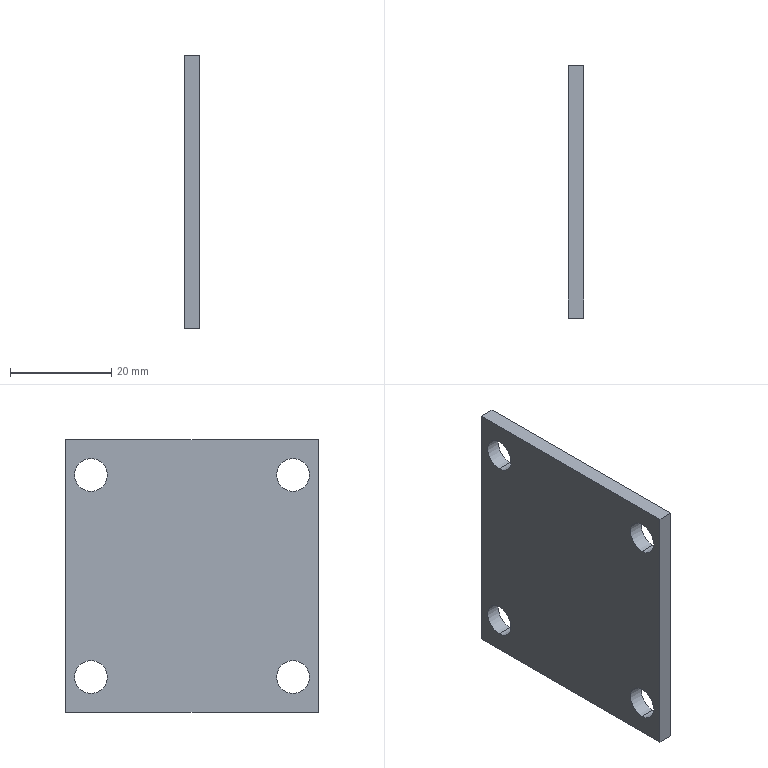Part | STEP file | 09-34 Linear bearing shim | 1 solid | 14 faces | box 3 x 50 x 54 mm | volume 7702 mm3 | cylinder 8 | plane 6 | commonest cylinder face diameters 6.5 x8
STEP:
#1=CARTESIAN_POINT('',(0.,0.,0.));
#2=DIRECTION('',(0.,0.,1.));
#3=DIRECTION('',(1.,0.,0.));
#4=AXIS2_PLACEMENT_3D('',#1,#2,#3);
#5=CARTESIAN_POINT('',(3.,-20.,23.25));
#6=VERTEX_POINT('',#5);
#7=CARTESIAN_POINT('',(0.,-20.,23.25));
#8=VERTEX_POINT('',#7);
#9=CARTESIAN_POINT('',(3.,-20.,23.25));
#10=DIRECTION('',(-1.,0.,0.));
#11=VECTOR('',#10,1.);
#12=LINE('',#9,#11);
#13=CARTESIAN_POINT('',(3.,-20.,20.));
#14=DIRECTION('',(-1.,0.,0.));
#15=DIRECTION('',(0.,0.,1.));
#16=AXIS2_PLACEMENT_3D('',#13,#14,#15);
#17=CYLINDRICAL_SURFACE('',#16,3.25);
#18=CARTESIAN_POINT('',(6.283,0.));
#19=DIRECTION('',(0.,1.));
#20=VECTOR('',#19,1.);
#21=LINE('',#18,#20);
#22=(GEOMETRIC_REPRESENTATION_CONTEXT(2)PARAMETRIC_REPRESENTATION_CONTEXT()REPRESENTATION_CONTEXT('',''));
#23=DEFINITIONAL_REPRESENTATION('',(#21),#22);
#24=PCURVE('',#17,#23);
#25=CARTESIAN_POINT('',(3.,-20.,20.));
#26=DIRECTION('',(-1.,0.,0.));
#27=DIRECTION('',(0.,0.,1.));
#28=AXIS2_PLACEMENT_3D('',#25,#26,#27);
#29=CYLINDRICAL_SURFACE('',#28,3.25);
#30=CARTESIAN_POINT('',(0.,0.));
#31=DIRECTION('',(0.,1.));
#32=VECTOR('',#31,1.);
#33=LINE('',#30,#32);
#34=(GEOMETRIC_REPRESENTATION_CONTEXT(2)PARAMETRIC_REPRESENTATION_CONTEXT()REPRESENTATION_CONTEXT('',''));
#35=DEFINITIONAL_REPRESENTATION('',(#33),#34);
#36=PCURVE('',#29,#35);
#37=SURFACE_CURVE('',#12,(#24,#36),.PCURVE_S1.);
#38=EDGE_CURVE('',#6,#8,#37,.T.);
#39=ORIENTED_EDGE('',*,*,#38,.T.);
#40=CARTESIAN_POINT('',(0.,-20.,16.75));
#41=VERTEX_POINT('',#40);
#42=CARTESIAN_POINT('',(0.,-20.,20.));
#43=DIRECTION('',(-1.,0.,0.));
#44=DIRECTION('',(0.,0.,1.));
#45=AXIS2_PLACEMENT_3D('',#42,#43,#44);
#46=CIRCLE('',#45,3.25);
#47=CARTESIAN_POINT('',(0.,3.));
#48=DIRECTION('',(1.,0.));
#49=VECTOR('',#48,1.);
#50=LINE('',#47,#49);
#51=(GEOMETRIC_REPRESENTATION_CONTEXT(2)PARAMETRIC_REPRESENTATION_CONTEXT()REPRESENTATION_CONTEXT('',''));
#52=DEFINITIONAL_REPRESENTATION('',(#50),#51);
#53=PCURVE('',#17,#52);
#54=CARTESIAN_POINT('',(0.,-25.,27.));
#55=DIRECTION('',(1.,0.,0.));
#56=DIRECTION('',(0.,0.,-1.));
#57=AXIS2_PLACEMENT_3D('',#54,#55,#56);
#58=PLANE('',#57);
#59=CARTESIAN_POINT('',(3.75,5.));
#60=CARTESIAN_POINT('',(3.75,10.629));
#61=CARTESIAN_POINT('',(8.625,7.815));
#62=CARTESIAN_POINT('',(13.5,5.));
#63=CARTESIAN_POINT('',(8.625,2.185));
#64=CARTESIAN_POINT('',(3.75,-0.6292));
#65=CARTESIAN_POINT('',(3.75,5.));
#66=(BOUNDED_CURVE()B_SPLINE_CURVE(2,(#59,#60,#61,#62,#63,#64,#65),.UNSPECIFIED.,.T.,.F.)B_SPLINE_CURVE_WITH_KNOTS((1,2,2,2,2,1),(-2.094,0.,2.094,4.189,6.283,8.378),.UNSPECIFIED.)CURVE()GEOMETRIC_REPRESENTATION_ITEM()RATIONAL_B_SPLINE_CURVE((1.,0.5,1.,0.5,1.,0.5,1.))REPRESENTATION_ITEM(''));
#67=(GEOMETRIC_REPRESENTATION_CONTEXT(2)PARAMETRIC_REPRESENTATION_CONTEXT()REPRESENTATION_CONTEXT('',''));
#68=DEFINITIONAL_REPRESENTATION('',(#66),#67);
#69=PCURVE('',#58,#68);
#70=SURFACE_CURVE('',#46,(#53,#69),.PCURVE_S1.);
#71=EDGE_CURVE('',#41,#8,#70,.T.);
#72=ORIENTED_EDGE('',*,*,#71,.F.);
#73=CARTESIAN_POINT('',(3.,-20.,16.75));
#74=VERTEX_POINT('',#73);
#75=CARTESIAN_POINT('',(3.,-20.,16.75));
#76=DIRECTION('',(-1.,0.,0.));
#77=VECTOR('',#76,1.);
#78=LINE('',#75,#77);
#79=CARTESIAN_POINT('',(3.142,0.));
#80=DIRECTION('',(0.,1.));
#81=VECTOR('',#80,1.);
#82=LINE('',#79,#81);
#83=(GEOMETRIC_REPRESENTATION_CONTEXT(2)PARAMETRIC_REPRESENTATION_CONTEXT()REPRESENTATION_CONTEXT('',''));
#84=DEFINITIONAL_REPRESENTATION('',(#82),#83);
#85=PCURVE('',#17,#84);
#86=CARTESIAN_POINT('',(3.142,0.));
#87=DIRECTION('',(0.,1.));
#88=VECTOR('',#87,1.);
#89=LINE('',#86,#88);
#90=(GEOMETRIC_REPRESENTATION_CONTEXT(2)PARAMETRIC_REPRESENTATION_CONTEXT()REPRESENTATION_CONTEXT('',''));
#91=DEFINITIONAL_REPRESENTATION('',(#89),#90);
#92=PCURVE('',#29,#91);
#93=SURFACE_CURVE('',#78,(#85,#92),.PCURVE_S1.);
#94=EDGE_CURVE('',#74,#41,#93,.T.);
#95=ORIENTED_EDGE('',*,*,#94,.F.);
#96=CARTESIAN_POINT('',(3.,-20.,20.));
#97=DIRECTION('',(1.,0.,0.));
#98=DIRECTION('',(0.,0.,1.));
#99=AXIS2_PLACEMENT_3D('',#96,#97,#98);
#100=CIRCLE('',#99,3.25);
#101=CARTESIAN_POINT('',(6.283,0.));
#102=DIRECTION('',(-1.,0.));
#103=VECTOR('',#102,1.);
#104=LINE('',#101,#103);
#105=(GEOMETRIC_REPRESENTATION_CONTEXT(2)PARAMETRIC_REPRESENTATION_CONTEXT()REPRESENTATION_CONTEXT('',''));
#106=DEFINITIONAL_REPRESENTATION('',(#104),#105);
#107=PCURVE('',#17,#106);
#108=CARTESIAN_POINT('',(3.,-25.,27.));
#109=DIRECTION('',(1.,0.,0.));
#110=DIRECTION('',(0.,0.,-1.));
#111=AXIS2_PLACEMENT_3D('',#108,#109,#110);
#112=PLANE('',#111);
#113=CARTESIAN_POINT('',(7.,5.));
#114=DIRECTION('',(-1.,0.));
#115=AXIS2_PLACEMENT_2D('',#113,#114);
#116=CIRCLE('',#115,3.25);
#117=(GEOMETRIC_REPRESENTATION_CONTEXT(2)PARAMETRIC_REPRESENTATION_CONTEXT()REPRESENTATION_CONTEXT('',''));
#118=DEFINITIONAL_REPRESENTATION('',(#116),#117);
#119=PCURVE('',#112,#118);
#120=SURFACE_CURVE('',#100,(#107,#119),.PCURVE_S1.);
#121=EDGE_CURVE('',#6,#74,#120,.T.);
#122=ORIENTED_EDGE('',*,*,#121,.F.);
#123=EDGE_LOOP('',(#39,#72,#95,#122));
#124=FACE_BOUND('',#123,.F.);
#125=ADVANCED_FACE('',(#124),#17,.F.);
#126=CARTESIAN_POINT('',(3.,20.,23.25));
#127=VERTEX_POINT('',#126);
#128=CARTESIAN_POINT('',(0.,20.,23.25));
#129=VERTEX_POINT('',#128);
#130=CARTESIAN_POINT('',(3.,20.,23.25));
#131=DIRECTION('',(-1.,0.,0.));
#132=VECTOR('',#131,1.);
#133=LINE('',#130,#132);
#134=CARTESIAN_POINT('',(3.,20.,20.));
#135=DIRECTION('',(-1.,0.,0.));
#136=DIRECTION('',(0.,0.,1.));
#137=AXIS2_PLACEMENT_3D('',#134,#135,#136);
#138=CYLINDRICAL_SURFACE('',#137,3.25);
#139=CARTESIAN_POINT('',(6.283,0.));
#140=DIRECTION('',(0.,1.));
#141=VECTOR('',#140,1.);
#142=LINE('',#139,#141);
#143=(GEOMETRIC_REPRESENTATION_CONTEXT(2)PARAMETRIC_REPRESENTATION_CONTEXT()REPRESENTATION_CONTEXT('',''));
#144=DEFINITIONAL_REPRESENTATION('',(#142),#143);
#145=PCURVE('',#138,#144);
#146=CARTESIAN_POINT('',(3.,20.,20.));
#147=DIRECTION('',(-1.,0.,0.));
#148=DIRECTION('',(0.,0.,1.));
#149=AXIS2_PLACEMENT_3D('',#146,#147,#148);
#150=CYLINDRICAL_SURFACE('',#149,3.25);
#151=CARTESIAN_POINT('',(0.,0.));
#152=DIRECTION('',(0.,1.));
#153=VECTOR('',#152,1.);
#154=LINE('',#151,#153);
#155=(GEOMETRIC_REPRESENTATION_CONTEXT(2)PARAMETRIC_REPRESENTATION_CONTEXT()REPRESENTATION_CONTEXT('',''));
#156=DEFINITIONAL_REPRESENTATION('',(#154),#155);
#157=PCURVE('',#150,#156);
#158=SURFACE_CURVE('',#133,(#145,#157),.PCURVE_S1.);
#159=EDGE_CURVE('',#127,#129,#158,.T.);
#160=ORIENTED_EDGE('',*,*,#159,.T.);
#161=CARTESIAN_POINT('',(0.,20.,16.75));
#162=VERTEX_POINT('',#161);
#163=CARTESIAN_POINT('',(0.,20.,20.));
#164=DIRECTION('',(-1.,0.,0.));
#165=DIRECTION('',(0.,0.,1.));
#166=AXIS2_PLACEMENT_3D('',#163,#164,#165);
#167=CIRCLE('',#166,3.25);
#168=CARTESIAN_POINT('',(0.,3.));
#169=DIRECTION('',(1.,0.));
#170=VECTOR('',#169,1.);
#171=LINE('',#168,#170);
#172=(GEOMETRIC_REPRESENTATION_CONTEXT(2)PARAMETRIC_REPRESENTATION_CONTEXT()REPRESENTATION_CONTEXT('',''));
#173=DEFINITIONAL_REPRESENTATION('',(#171),#172);
#174=PCURVE('',#138,#173);
#175=CARTESIAN_POINT('',(3.75,45.));
#176=CARTESIAN_POINT('',(3.75,50.629));
#177=CARTESIAN_POINT('',(8.625,47.815));
#178=CARTESIAN_POINT('',(13.5,45.));
#179=CARTESIAN_POINT('',(8.625,42.185));
#180=CARTESIAN_POINT('',(3.75,39.371));
#181=CARTESIAN_POINT('',(3.75,45.));
#182=(BOUNDED_CURVE()B_SPLINE_CURVE(2,(#175,#176,#177,#178,#179,#180,#181),.UNSPECIFIED.,.T.,.F.)B_SPLINE_CURVE_WITH_KNOTS((1,2,2,2,2,1),(-2.094,0.,2.094,4.189,6.283,8.378),.UNSPECIFIED.)CURVE()GEOMETRIC_REPRESENTATION_ITEM()RATIONAL_B_SPLINE_CURVE((1.,0.5,1.,0.5,1.,0.5,1.))REPRESENTATION_ITEM(''));
#183=(GEOMETRIC_REPRESENTATION_CONTEXT(2)PARAMETRIC_REPRESENTATION_CONTEXT()REPRESENTATION_CONTEXT('',''));
#184=DEFINITIONAL_REPRESENTATION('',(#182),#183);
#185=PCURVE('',#58,#184);
#186=SURFACE_CURVE('',#167,(#174,#185),.PCURVE_S1.);
#187=EDGE_CURVE('',#162,#129,#186,.T.);
#188=ORIENTED_EDGE('',*,*,#187,.F.);
#189=CARTESIAN_POINT('',(3.,20.,16.75));
#190=VERTEX_POINT('',#189);
#191=CARTESIAN_POINT('',(3.,20.,16.75));
#192=DIRECTION('',(-1.,0.,0.));
#193=VECTOR('',#192,1.);
#194=LINE('',#191,#193);
#195=CARTESIAN_POINT('',(3.142,0.));
#196=DIRECTION('',(0.,1.));
#197=VECTOR('',#196,1.);
#198=LINE('',#195,#197);
#199=(GEOMETRIC_REPRESENTATION_CONTEXT(2)PARAMETRIC_REPRESENTATION_CONTEXT()REPRESENTATION_CONTEXT('',''));
#200=DEFINITIONAL_REPRESENTATION('',(#198),#199);
#201=PCURVE('',#138,#200);
#202=CARTESIAN_POINT('',(3.142,0.));
#203=DIRECTION('',(0.,1.));
#204=VECTOR('',#203,1.);
#205=LINE('',#202,#204);
#206=(GEOMETRIC_REPRESENTATION_CONTEXT(2)PARAMETRIC_REPRESENTATION_CONTEXT()REPRESENTATION_CONTEXT('',''));
#207=DEFINITIONAL_REPRESENTATION('',(#205),#206);
#208=PCURVE('',#150,#207);
#209=SURFACE_CURVE('',#194,(#201,#208),.PCURVE_S1.);
#210=EDGE_CURVE('',#190,#162,#209,.T.);
#211=ORIENTED_EDGE('',*,*,#210,.F.);
#212=CARTESIAN_POINT('',(3.,20.,20.));
#213=DIRECTION('',(-1.,0.,0.));
#214=DIRECTION('',(0.,0.,1.));
#215=AXIS2_PLACEMENT_3D('',#212,#213,#214);
#216=CIRCLE('',#215,3.25);
#217=CARTESIAN_POINT('',(0.,0.));
#218=DIRECTION('',(1.,0.));
#219=VECTOR('',#218,1.);
#220=LINE('',#217,#219);
#221=(GEOMETRIC_REPRESENTATION_CONTEXT(2)PARAMETRIC_REPRESENTATION_CONTEXT()REPRESENTATION_CONTEXT('',''));
#222=DEFINITIONAL_REPRESENTATION('',(#220),#221);
#223=PCURVE('',#138,#222);
#224=CARTESIAN_POINT('',(3.75,45.));
#225=CARTESIAN_POINT('',(3.75,50.629));
#226=CARTESIAN_POINT('',(8.625,47.815));
#227=CARTESIAN_POINT('',(13.5,45.));
#228=CARTESIAN_POINT('',(8.625,42.185));
#229=CARTESIAN_POINT('',(3.75,39.371));
#230=CARTESIAN_POINT('',(3.75,45.));
#231=(BOUNDED_CURVE()B_SPLINE_CURVE(2,(#224,#225,#226,#227,#228,#229,#230),.UNSPECIFIED.,.T.,.F.)B_SPLINE_CURVE_WITH_KNOTS((1,2,2,2,2,1),(-2.094,0.,2.094,4.189,6.283,8.378),.UNSPECIFIED.)CURVE()GEOMETRIC_REPRESENTATION_ITEM()RATIONAL_B_SPLINE_CURVE((1.,0.5,1.,0.5,1.,0.5,1.))REPRESENTATION_ITEM(''));
#232=(GEOMETRIC_REPRESENTATION_CONTEXT(2)PARAMETRIC_REPRESENTATION_CONTEXT()REPRESENTATION_CONTEXT('',''));
#233=DEFINITIONAL_REPRESENTATION('',(#231),#232);
#234=PCURVE('',#112,#233);
#235=SURFACE_CURVE('',#216,(#223,#234),.PCURVE_S1.);
#236=EDGE_CURVE('',#190,#127,#235,.T.);
#237=ORIENTED_EDGE('',*,*,#236,.T.);
#238=EDGE_LOOP('',(#160,#188,#211,#237));
#239=FACE_BOUND('',#238,.F.);
#240=ADVANCED_FACE('',(#239),#138,.F.);
#241=CARTESIAN_POINT('',(3.,20.,-16.75));
#242=VERTEX_POINT('',#241);
#243=CARTESIAN_POINT('',(0.,20.,-16.75));
#244=VERTEX_POINT('',#243);
#245=CARTESIAN_POINT('',(3.,20.,-16.75));
#246=DIRECTION('',(-1.,0.,0.));
#247=VECTOR('',#246,1.);
#248=LINE('',#245,#247);
#249=CARTESIAN_POINT('',(3.,20.,-20.));
#250=DIRECTION('',(-1.,0.,0.));
#251=DIRECTION('',(0.,0.,1.));
#252=AXIS2_PLACEMENT_3D('',#249,#250,#251);
#253=CYLINDRICAL_SURFACE('',#252,3.25);
#254=CARTESIAN_POINT('',(6.283,0.));
#255=DIRECTION('',(0.,1.));
#256=VECTOR('',#255,1.);
#257=LINE('',#254,#256);
#258=(GEOMETRIC_REPRESENTATION_CONTEXT(2)PARAMETRIC_REPRESENTATION_CONTEXT()REPRESENTATION_CONTEXT('',''));
#259=DEFINITIONAL_REPRESENTATION('',(#257),#258);
#260=PCURVE('',#253,#259);
#261=CARTESIAN_POINT('',(3.,20.,-20.));
#262=DIRECTION('',(-1.,0.,0.));
#263=DIRECTION('',(0.,0.,1.));
#264=AXIS2_PLACEMENT_3D('',#261,#262,#263);
#265=CYLINDRICAL_SURFACE('',#264,3.25);
#266=CARTESIAN_POINT('',(0.,0.));
#267=DIRECTION('',(0.,1.));
#268=VECTOR('',#267,1.);
#269=LINE('',#266,#268);
#270=(GEOMETRIC_REPRESENTATION_CONTEXT(2)PARAMETRIC_REPRESENTATION_CONTEXT()REPRESENTATION_CONTEXT('',''));
#271=DEFINITIONAL_REPRESENTATION('',(#269),#270);
#272=PCURVE('',#265,#271);
#273=SURFACE_CURVE('',#248,(#260,#272),.PCURVE_S1.);
#274=EDGE_CURVE('',#242,#244,#273,.T.);
#275=ORIENTED_EDGE('',*,*,#274,.T.);
#276=CARTESIAN_POINT('',(0.,20.,-23.25));
#277=VERTEX_POINT('',#276);
#278=CARTESIAN_POINT('',(0.,20.,-20.));
#279=DIRECTION('',(-1.,0.,0.));
#280=DIRECTION('',(0.,0.,1.));
#281=AXIS2_PLACEMENT_3D('',#278,#279,#280);
#282=CIRCLE('',#281,3.25);
#283=CARTESIAN_POINT('',(0.,3.));
#284=DIRECTION('',(1.,0.));
#285=VECTOR('',#284,1.);
#286=LINE('',#283,#285);
#287=(GEOMETRIC_REPRESENTATION_CONTEXT(2)PARAMETRIC_REPRESENTATION_CONTEXT()REPRESENTATION_CONTEXT('',''));
#288=DEFINITIONAL_REPRESENTATION('',(#286),#287);
#289=PCURVE('',#253,#288);
#290=CARTESIAN_POINT('',(43.75,45.));
#291=CARTESIAN_POINT('',(43.75,50.629));
#292=CARTESIAN_POINT('',(48.625,47.815));
#293=CARTESIAN_POINT('',(53.5,45.));
#294=CARTESIAN_POINT('',(48.625,42.185));
#295=CARTESIAN_POINT('',(43.75,39.371));
#296=CARTESIAN_POINT('',(43.75,45.));
#297=(BOUNDED_CURVE()B_SPLINE_CURVE(2,(#290,#291,#292,#293,#294,#295,#296),.UNSPECIFIED.,.T.,.F.)B_SPLINE_CURVE_WITH_KNOTS((1,2,2,2,2,1),(-2.094,0.,2.094,4.189,6.283,8.378),.UNSPECIFIED.)CURVE()GEOMETRIC_REPRESENTATION_ITEM()RATIONAL_B_SPLINE_CURVE((1.,0.5,1.,0.5,1.,0.5,1.))REPRESENTATION_ITEM(''));
#298=(GEOMETRIC_REPRESENTATION_CONTEXT(2)PARAMETRIC_REPRESENTATION_CONTEXT()REPRESENTATION_CONTEXT('',''));
#299=DEFINITIONAL_REPRESENTATION('',(#297),#298);
#300=PCURVE('',#58,#299);
#301=SURFACE_CURVE('',#282,(#289,#300),.PCURVE_S1.);
#302=EDGE_CURVE('',#277,#244,#301,.T.);
#303=ORIENTED_EDGE('',*,*,#302,.F.);
#304=CARTESIAN_POINT('',(3.,20.,-23.25));
#305=VERTEX_POINT('',#304);
#306=CARTESIAN_POINT('',(3.,20.,-23.25));
#307=DIRECTION('',(-1.,0.,0.));
#308=VECTOR('',#307,1.);
#309=LINE('',#306,#308);
#310=CARTESIAN_POINT('',(3.142,0.));
#311=DIRECTION('',(0.,1.));
#312=VECTOR('',#311,1.);
#313=LINE('',#310,#312);
#314=(GEOMETRIC_REPRESENTATION_CONTEXT(2)PARAMETRIC_REPRESENTATION_CONTEXT()REPRESENTATION_CONTEXT('',''));
#315=DEFINITIONAL_REPRESENTATION('',(#313),#314);
#316=PCURVE('',#253,#315);
#317=CARTESIAN_POINT('',(3.142,0.));
#318=DIRECTION('',(0.,1.));
#319=VECTOR('',#318,1.);
#320=LINE('',#317,#319);
#321=(GEOMETRIC_REPRESENTATION_CONTEXT(2)PARAMETRIC_REPRESENTATION_CONTEXT()REPRESENTATION_CONTEXT('',''));
#322=DEFINITIONAL_REPRESENTATION('',(#320),#321);
#323=PCURVE('',#265,#322);
#324=SURFACE_CURVE('',#309,(#316,#323),.PCURVE_S1.);
#325=EDGE_CURVE('',#305,#277,#324,.T.);
#326=ORIENTED_EDGE('',*,*,#325,.F.);
#327=CARTESIAN_POINT('',(3.,20.,-20.));
#328=DIRECTION('',(-1.,0.,0.));
#329=DIRECTION('',(0.,0.,1.));
#330=AXIS2_PLACEMENT_3D('',#327,#328,#329);
#331=CIRCLE('',#330,3.25);
#332=CARTESIAN_POINT('',(0.,0.));
#333=DIRECTION('',(1.,0.));
#334=VECTOR('',#333,1.);
#335=LINE('',#332,#334);
#336=(GEOMETRIC_REPRESENTATION_CONTEXT(2)PARAMETRIC_REPRESENTATION_CONTEXT()REPRESENTATION_CONTEXT('',''));
#337=DEFINITIONAL_REPRESENTATION('',(#335),#336);
#338=PCURVE('',#253,#337);
#339=CARTESIAN_POINT('',(43.75,45.));
#340=CARTESIAN_POINT('',(43.75,50.629));
#341=CARTESIAN_POINT('',(48.625,47.815));
#342=CARTESIAN_POINT('',(53.5,45.));
#343=CARTESIAN_POINT('',(48.625,42.185));
#344=CARTESIAN_POINT('',(43.75,39.371));
#345=CARTESIAN_POINT('',(43.75,45.));
#346=(BOUNDED_CURVE()B_SPLINE_CURVE(2,(#339,#340,#341,#342,#343,#344,#345),.UNSPECIFIED.,.T.,.F.)B_SPLINE_CURVE_WITH_KNOTS((1,2,2,2,2,1),(-2.094,0.,2.094,4.189,6.283,8.378),.UNSPECIFIED.)CURVE()GEOMETRIC_REPRESENTATION_ITEM()RATIONAL_B_SPLINE_CURVE((1.,0.5,1.,0.5,1.,0.5,1.))REPRESENTATION_ITEM(''));
#347=(GEOMETRIC_REPRESENTATION_CONTEXT(2)PARAMETRIC_REPRESENTATION_CONTEXT()REPRESENTATION_CONTEXT('',''));
#348=DEFINITIONAL_REPRESENTATION('',(#346),#347);
#349=PCURVE('',#112,#348);
#350=SURFACE_CURVE('',#331,(#338,#349),.PCURVE_S1.);
#351=EDGE_CURVE('',#305,#242,#350,.T.);
#352=ORIENTED_EDGE('',*,*,#351,.T.);
#353=EDGE_LOOP('',(#275,#303,#326,#352));
#354=FACE_BOUND('',#353,.F.);
#355=ADVANCED_FACE('',(#354),#253,.F.);
#356=CARTESIAN_POINT('',(3.,-20.,-16.75));
#357=VERTEX_POINT('',#356);
#358=CARTESIAN_POINT('',(0.,-20.,-16.75));
#359=VERTEX_POINT('',#358);
#360=CARTESIAN_POINT('',(3.,-20.,-16.75));
#361=DIRECTION('',(-1.,0.,0.));
#362=VECTOR('',#361,1.);
#363=LINE('',#360,#362);
#364=CARTESIAN_POINT('',(3.,-20.,-20.));
#365=DIRECTION('',(-1.,0.,0.));
#366=DIRECTION('',(0.,0.,1.));
#367=AXIS2_PLACEMENT_3D('',#364,#365,#366);
#368=CYLINDRICAL_SURFACE('',#367,3.25);
#369=CARTESIAN_POINT('',(6.283,0.));
#370=DIRECTION('',(0.,1.));
#371=VECTOR('',#370,1.);
#372=LINE('',#369,#371);
#373=(GEOMETRIC_REPRESENTATION_CONTEXT(2)PARAMETRIC_REPRESENTATION_CONTEXT()REPRESENTATION_CONTEXT('',''));
#374=DEFINITIONAL_REPRESENTATION('',(#372),#373);
#375=PCURVE('',#368,#374);
#376=CARTESIAN_POINT('',(3.,-20.,-20.));
#377=DIRECTION('',(-1.,0.,0.));
#378=DIRECTION('',(0.,0.,1.));
#379=AXIS2_PLACEMENT_3D('',#376,#377,#378);
#380=CYLINDRICAL_SURFACE('',#379,3.25);
#381=CARTESIAN_POINT('',(0.,0.));
#382=DIRECTION('',(0.,1.));
#383=VECTOR('',#382,1.);
#384=LINE('',#381,#383);
#385=(GEOMETRIC_REPRESENTATION_CONTEXT(2)PARAMETRIC_REPRESENTATION_CONTEXT()REPRESENTATION_CONTEXT('',''));
#386=DEFINITIONAL_REPRESENTATION('',(#384),#385);
#387=PCURVE('',#380,#386);
#388=SURFACE_CURVE('',#363,(#375,#387),.PCURVE_S1.);
#389=EDGE_CURVE('',#357,#359,#388,.T.);
#390=ORIENTED_EDGE('',*,*,#389,.T.);
#391=CARTESIAN_POINT('',(0.,-20.,-23.25));
#392=VERTEX_POINT('',#391);
#393=CARTESIAN_POINT('',(0.,-20.,-20.));
#394=DIRECTION('',(-1.,0.,0.));
#395=DIRECTION('',(0.,0.,1.));
#396=AXIS2_PLACEMENT_3D('',#393,#394,#395);
#397=CIRCLE('',#396,3.25);
#398=CARTESIAN_POINT('',(0.,3.));
#399=DIRECTION('',(1.,0.));
#400=VECTOR('',#399,1.);
#401=LINE('',#398,#400);
#402=(GEOMETRIC_REPRESENTATION_CONTEXT(2)PARAMETRIC_REPRESENTATION_CONTEXT()REPRESENTATION_CONTEXT('',''));
#403=DEFINITIONAL_REPRESENTATION('',(#401),#402);
#404=PCURVE('',#368,#403);
#405=CARTESIAN_POINT('',(43.75,5.));
#406=CARTESIAN_POINT('',(43.75,10.629));
#407=CARTESIAN_POINT('',(48.625,7.815));
#408=CARTESIAN_POINT('',(53.5,5.));
#409=CARTESIAN_POINT('',(48.625,2.185));
#410=CARTESIAN_POINT('',(43.75,-0.6292));
#411=CARTESIAN_POINT('',(43.75,5.));
#412=(BOUNDED_CURVE()B_SPLINE_CURVE(2,(#405,#406,#407,#408,#409,#410,#411),.UNSPECIFIED.,.T.,.F.)B_SPLINE_CURVE_WITH_KNOTS((1,2,2,2,2,1),(-2.094,0.,2.094,4.189,6.283,8.378),.UNSPECIFIED.)CURVE()GEOMETRIC_REPRESENTATION_ITEM()RATIONAL_B_SPLINE_CURVE((1.,0.5,1.,0.5,1.,0.5,1.))REPRESENTATION_ITEM(''));
#413=(GEOMETRIC_REPRESENTATION_CONTEXT(2)PARAMETRIC_REPRESENTATION_CONTEXT()REPRESENTATION_CONTEXT('',''));
#414=DEFINITIONAL_REPRESENTATION('',(#412),#413);
#415=PCURVE('',#58,#414);
#416=SURFACE_CURVE('',#397,(#404,#415),.PCURVE_S1.);
#417=EDGE_CURVE('',#392,#359,#416,.T.);
#418=ORIENTED_EDGE('',*,*,#417,.F.);
#419=CARTESIAN_POINT('',(3.,-20.,-23.25));
#420=VERTEX_POINT('',#419);
#421=CARTESIAN_POINT('',(3.,-20.,-23.25));
#422=DIRECTION('',(-1.,0.,0.));
#423=VECTOR('',#422,1.);
#424=LINE('',#421,#423);
#425=CARTESIAN_POINT('',(3.142,0.));
#426=DIRECTION('',(0.,1.));
#427=VECTOR('',#426,1.);
#428=LINE('',#425,#427);
#429=(GEOMETRIC_REPRESENTATION_CONTEXT(2)PARAMETRIC_REPRESENTATION_CONTEXT()REPRESENTATION_CONTEXT('',''));
#430=DEFINITIONAL_REPRESENTATION('',(#428),#429);
#431=PCURVE('',#368,#430);
#432=CARTESIAN_POINT('',(3.142,0.));
#433=DIRECTION('',(0.,1.));
#434=VECTOR('',#433,1.);
#435=LINE('',#432,#434);
#436=(GEOMETRIC_REPRESENTATION_CONTEXT(2)PARAMETRIC_REPRESENTATION_CONTEXT()REPRESENTATION_CONTEXT('',''));
#437=DEFINITIONAL_REPRESENTATION('',(#435),#436);
#438=PCURVE('',#380,#437);
#439=SURFACE_CURVE('',#424,(#431,#438),.PCURVE_S1.);
#440=EDGE_CURVE('',#420,#392,#439,.T.);
#441=ORIENTED_EDGE('',*,*,#440,.F.);
#442=CARTESIAN_POINT('',(3.,-20.,-20.));
#443=DIRECTION('',(-1.,0.,0.));
#444=DIRECTION('',(0.,0.,1.));
#445=AXIS2_PLACEMENT_3D('',#442,#443,#444);
#446=CIRCLE('',#445,3.25);
#447=CARTESIAN_POINT('',(0.,0.));
#448=DIRECTION('',(1.,0.));
#449=VECTOR('',#448,1.);
#450=LINE('',#447,#449);
#451=(GEOMETRIC_REPRESENTATION_CONTEXT(2)PARAMETRIC_REPRESENTATION_CONTEXT()REPRESENTATION_CONTEXT('',''));
#452=DEFINITIONAL_REPRESENTATION('',(#450),#451);
#453=PCURVE('',#368,#452);
#454=CARTESIAN_POINT('',(43.75,5.));
#455=CARTESIAN_POINT('',(43.75,10.629));
#456=CARTESIAN_POINT('',(48.625,7.815));
#457=CARTESIAN_POINT('',(53.5,5.));
#458=CARTESIAN_POINT('',(48.625,2.185));
#459=CARTESIAN_POINT('',(43.75,-0.6292));
#460=CARTESIAN_POINT('',(43.75,5.));
#461=(BOUNDED_CURVE()B_SPLINE_CURVE(2,(#454,#455,#456,#457,#458,#459,#460),.UNSPECIFIED.,.T.,.F.)B_SPLINE_CURVE_WITH_KNOTS((1,2,2,2,2,1),(-2.094,0.,2.094,4.189,6.283,8.378),.UNSPECIFIED.)CURVE()GEOMETRIC_REPRESENTATION_ITEM()RATIONAL_B_SPLINE_CURVE((1.,0.5,1.,0.5,1.,0.5,1.))REPRESENTATION_ITEM(''));
#462=(GEOMETRIC_REPRESENTATION_CONTEXT(2)PARAMETRIC_REPRESENTATION_CONTEXT()REPRESENTATION_CONTEXT('',''));
#463=DEFINITIONAL_REPRESENTATION('',(#461),#462);
#464=PCURVE('',#112,#463);
#465=SURFACE_CURVE('',#446,(#453,#464),.PCURVE_S1.);
#466=EDGE_CURVE('',#420,#357,#465,.T.);
#467=ORIENTED_EDGE('',*,*,#466,.T.);
#468=EDGE_LOOP('',(#390,#418,#441,#467));
#469=FACE_BOUND('',#468,.F.);
#470=ADVANCED_FACE('',(#469),#368,.F.);
#471=CARTESIAN_POINT('',(0.,-20.,20.));
#472=DIRECTION('',(-1.,0.,0.));
#473=DIRECTION('',(0.,0.,1.));
#474=AXIS2_PLACEMENT_3D('',#471,#472,#473);
#475=CIRCLE('',#474,3.25);
#476=CARTESIAN_POINT('',(0.,3.));
#477=DIRECTION('',(1.,0.));
#478=VECTOR('',#477,1.);
#479=LINE('',#476,#478);
#480=(GEOMETRIC_REPRESENTATION_CONTEXT(2)PARAMETRIC_REPRESENTATION_CONTEXT()REPRESENTATION_CONTEXT('',''));
#481=DEFINITIONAL_REPRESENTATION('',(#479),#480);
#482=PCURVE('',#29,#481);
#483=CARTESIAN_POINT('',(3.75,5.));
#484=CARTESIAN_POINT('',(3.75,10.629));
#485=CARTESIAN_POINT('',(8.625,7.815));
#486=CARTESIAN_POINT('',(13.5,5.));
#487=CARTESIAN_POINT('',(8.625,2.185));
#488=CARTESIAN_POINT('',(3.75,-0.6292));
#489=CARTESIAN_POINT('',(3.75,5.));
#490=(BOUNDED_CURVE()B_SPLINE_CURVE(2,(#483,#484,#485,#486,#487,#488,#489),.UNSPECIFIED.,.T.,.F.)B_SPLINE_CURVE_WITH_KNOTS((1,2,2,2,2,1),(-2.094,0.,2.094,4.189,6.283,8.378),.UNSPECIFIED.)CURVE()GEOMETRIC_REPRESENTATION_ITEM()RATIONAL_B_SPLINE_CURVE((1.,0.5,1.,0.5,1.,0.5,1.))REPRESENTATION_ITEM(''));
#491=(GEOMETRIC_REPRESENTATION_CONTEXT(2)PARAMETRIC_REPRESENTATION_CONTEXT()REPRESENTATION_CONTEXT('',''));
#492=DEFINITIONAL_REPRESENTATION('',(#490),#491);
#493=PCURVE('',#58,#492);
#494=SURFACE_CURVE('',#475,(#482,#493),.PCURVE_S1.);
#495=EDGE_CURVE('',#8,#41,#494,.T.);
#496=ORIENTED_EDGE('',*,*,#495,.F.);
#497=ORIENTED_EDGE('',*,*,#38,.F.);
#498=CARTESIAN_POINT('',(3.,-20.,20.));
#499=DIRECTION('',(1.,0.,0.));
#500=DIRECTION('',(0.,0.,1.));
#501=AXIS2_PLACEMENT_3D('',#498,#499,#500);
#502=CIRCLE('',#501,3.25);
#503=CARTESIAN_POINT('',(6.283,0.));
#504=DIRECTION('',(-1.,0.));
#505=VECTOR('',#504,1.);
#506=LINE('',#503,#505);
#507=(GEOMETRIC_REPRESENTATION_CONTEXT(2)PARAMETRIC_REPRESENTATION_CONTEXT()REPRESENTATION_CONTEXT('',''));
#508=DEFINITIONAL_REPRESENTATION('',(#506),#507);
#509=PCURVE('',#29,#508);
#510=CARTESIAN_POINT('',(7.,5.));
#511=DIRECTION('',(-1.,0.));
#512=AXIS2_PLACEMENT_2D('',#510,#511);
#513=CIRCLE('',#512,3.25);
#514=(GEOMETRIC_REPRESENTATION_CONTEXT(2)PARAMETRIC_REPRESENTATION_CONTEXT()REPRESENTATION_CONTEXT('',''));
#515=DEFINITIONAL_REPRESENTATION('',(#513),#514);
#516=PCURVE('',#112,#515);
#517=SURFACE_CURVE('',#502,(#509,#516),.PCURVE_S1.);
#518=EDGE_CURVE('',#74,#6,#517,.T.);
#519=ORIENTED_EDGE('',*,*,#518,.F.);
#520=ORIENTED_EDGE('',*,*,#94,.T.);
#521=EDGE_LOOP('',(#496,#497,#519,#520));
#522=FACE_BOUND('',#521,.F.);
#523=ADVANCED_FACE('',(#522),#29,.F.);
#524=ORIENTED_EDGE('',*,*,#495,.F.);
#525=ORIENTED_EDGE('',*,*,#71,.F.);
#526=EDGE_LOOP('',(#524,#525));
#527=FACE_BOUND('',#526,.T.);
#528=CARTESIAN_POINT('',(0.,20.,20.));
#529=DIRECTION('',(-1.,0.,0.));
#530=DIRECTION('',(0.,0.,1.));
#531=AXIS2_PLACEMENT_3D('',#528,#529,#530);
#532=CIRCLE('',#531,3.25);
#533=CARTESIAN_POINT('',(3.75,45.));
#534=CARTESIAN_POINT('',(3.75,50.629));
#535=CARTESIAN_POINT('',(8.625,47.815));
#536=CARTESIAN_POINT('',(13.5,45.));
#537=CARTESIAN_POINT('',(8.625,42.185));
#538=CARTESIAN_POINT('',(3.75,39.371));
#539=CARTESIAN_POINT('',(3.75,45.));
#540=(BOUNDED_CURVE()B_SPLINE_CURVE(2,(#533,#534,#535,#536,#537,#538,#539),.UNSPECIFIED.,.T.,.F.)B_SPLINE_CURVE_WITH_KNOTS((1,2,2,2,2,1),(-2.094,0.,2.094,4.189,6.283,8.378),.UNSPECIFIED.)CURVE()GEOMETRIC_REPRESENTATION_ITEM()RATIONAL_B_SPLINE_CURVE((1.,0.5,1.,0.5,1.,0.5,1.))REPRESENTATION_ITEM(''));
#541=(GEOMETRIC_REPRESENTATION_CONTEXT(2)PARAMETRIC_REPRESENTATION_CONTEXT()REPRESENTATION_CONTEXT('',''));
#542=DEFINITIONAL_REPRESENTATION('',(#540),#541);
#543=PCURVE('',#58,#542);
#544=CARTESIAN_POINT('',(0.,3.));
#545=DIRECTION('',(1.,0.));
#546=VECTOR('',#545,1.);
#547=LINE('',#544,#546);
#548=(GEOMETRIC_REPRESENTATION_CONTEXT(2)PARAMETRIC_REPRESENTATION_CONTEXT()REPRESENTATION_CONTEXT('',''));
#549=DEFINITIONAL_REPRESENTATION('',(#547),#548);
#550=PCURVE('',#150,#549);
#551=SURFACE_CURVE('',#532,(#543,#550),.PCURVE_S1.);
#552=EDGE_CURVE('',#129,#162,#551,.T.);
#553=ORIENTED_EDGE('',*,*,#552,.F.);
#554=ORIENTED_EDGE('',*,*,#187,.F.);
#555=EDGE_LOOP('',(#553,#554));
#556=FACE_BOUND('',#555,.T.);
#557=CARTESIAN_POINT('',(0.,20.,-20.));
#558=DIRECTION('',(-1.,0.,0.));
#559=DIRECTION('',(0.,0.,1.));
#560=AXIS2_PLACEMENT_3D('',#557,#558,#559);
#561=CIRCLE('',#560,3.25);
#562=CARTESIAN_POINT('',(43.75,45.));
#563=CARTESIAN_POINT('',(43.75,50.629));
#564=CARTESIAN_POINT('',(48.625,47.815));
#565=CARTESIAN_POINT('',(53.5,45.));
#566=CARTESIAN_POINT('',(48.625,42.185));
#567=CARTESIAN_POINT('',(43.75,39.371));
#568=CARTESIAN_POINT('',(43.75,45.));
#569=(BOUNDED_CURVE()B_SPLINE_CURVE(2,(#562,#563,#564,#565,#566,#567,#568),.UNSPECIFIED.,.T.,.F.)B_SPLINE_CURVE_WITH_KNOTS((1,2,2,2,2,1),(-2.094,0.,2.094,4.189,6.283,8.378),.UNSPECIFIED.)CURVE()GEOMETRIC_REPRESENTATION_ITEM()RATIONAL_B_SPLINE_CURVE((1.,0.5,1.,0.5,1.,0.5,1.))REPRESENTATION_ITEM(''));
#570=(GEOMETRIC_REPRESENTATION_CONTEXT(2)PARAMETRIC_REPRESENTATION_CONTEXT()REPRESENTATION_CONTEXT('',''));
#571=DEFINITIONAL_REPRESENTATION('',(#569),#570);
#572=PCURVE('',#58,#571);
#573=CARTESIAN_POINT('',(0.,3.));
#574=DIRECTION('',(1.,0.));
#575=VECTOR('',#574,1.);
#576=LINE('',#573,#575);
#577=(GEOMETRIC_REPRESENTATION_CONTEXT(2)PARAMETRIC_REPRESENTATION_CONTEXT()REPRESENTATION_CONTEXT('',''));
#578=DEFINITIONAL_REPRESENTATION('',(#576),#577);
#579=PCURVE('',#265,#578);
#580=SURFACE_CURVE('',#561,(#572,#579),.PCURVE_S1.);
#581=EDGE_CURVE('',#244,#277,#580,.T.);
#582=ORIENTED_EDGE('',*,*,#581,.F.);
#583=ORIENTED_EDGE('',*,*,#302,.F.);
#584=EDGE_LOOP('',(#582,#583));
#585=FACE_BOUND('',#584,.T.);
#586=CARTESIAN_POINT('',(0.,-20.,-20.));
#587=DIRECTION('',(-1.,0.,0.));
#588=DIRECTION('',(0.,0.,1.));
#589=AXIS2_PLACEMENT_3D('',#586,#587,#588);
#590=CIRCLE('',#589,3.25);
#591=CARTESIAN_POINT('',(43.75,5.));
#592=CARTESIAN_POINT('',(43.75,10.629));
#593=CARTESIAN_POINT('',(48.625,7.815));
#594=CARTESIAN_POINT('',(53.5,5.));
#595=CARTESIAN_POINT('',(48.625,2.185));
#596=CARTESIAN_POINT('',(43.75,-0.6292));
#597=CARTESIAN_POINT('',(43.75,5.));
#598=(BOUNDED_CURVE()B_SPLINE_CURVE(2,(#591,#592,#593,#594,#595,#596,#597),.UNSPECIFIED.,.T.,.F.)B_SPLINE_CURVE_WITH_KNOTS((1,2,2,2,2,1),(-2.094,0.,2.094,4.189,6.283,8.378),.UNSPECIFIED.)CURVE()GEOMETRIC_REPRESENTATION_ITEM()RATIONAL_B_SPLINE_CURVE((1.,0.5,1.,0.5,1.,0.5,1.))REPRESENTATION_ITEM(''));
#599=(GEOMETRIC_REPRESENTATION_CONTEXT(2)PARAMETRIC_REPRESENTATION_CONTEXT()REPRESENTATION_CONTEXT('',''));
#600=DEFINITIONAL_REPRESENTATION('',(#598),#599);
#601=PCURVE('',#58,#600);
#602=CARTESIAN_POINT('',(0.,3.));
#603=DIRECTION('',(1.,0.));
#604=VECTOR('',#603,1.);
#605=LINE('',#602,#604);
#606=(GEOMETRIC_REPRESENTATION_CONTEXT(2)PARAMETRIC_REPRESENTATION_CONTEXT()REPRESENTATION_CONTEXT('',''));
#607=DEFINITIONAL_REPRESENTATION('',(#605),#606);
#608=PCURVE('',#380,#607);
#609=SURFACE_CURVE('',#590,(#601,#608),.PCURVE_S1.);
#610=EDGE_CURVE('',#359,#392,#609,.T.);
#611=ORIENTED_EDGE('',*,*,#610,.F.);
#612=ORIENTED_EDGE('',*,*,#417,.F.);
#613=EDGE_LOOP('',(#611,#612));
#614=FACE_BOUND('',#613,.T.);
#615=CARTESIAN_POINT('',(0.,25.,-27.));
#616=VERTEX_POINT('',#615);
#617=CARTESIAN_POINT('',(0.,25.,27.));
#618=VERTEX_POINT('',#617);
#619=CARTESIAN_POINT('',(0.,25.,0.));
#620=DIRECTION('',(0.,0.,1.));
#621=VECTOR('',#620,1.);
#622=LINE('',#619,#621);
#623=CARTESIAN_POINT('',(27.,50.));
#624=DIRECTION('',(-1.,0.));
#625=VECTOR('',#624,1.);
#626=LINE('',#623,#625);
#627=(GEOMETRIC_REPRESENTATION_CONTEXT(2)PARAMETRIC_REPRESENTATION_CONTEXT()REPRESENTATION_CONTEXT('',''));
#628=DEFINITIONAL_REPRESENTATION('',(#626),#627);
#629=PCURVE('',#58,#628);
#630=CARTESIAN_POINT('',(0.,25.,27.));
#631=DIRECTION('',(0.,-1.,0.));
#632=DIRECTION('',(0.,0.,-1.));
#633=AXIS2_PLACEMENT_3D('',#630,#631,#632);
#634=PLANE('',#633);
#635=CARTESIAN_POINT('',(27.,0.));
#636=DIRECTION('',(-1.,0.));
#637=VECTOR('',#636,1.);
#638=LINE('',#635,#637);
#639=(GEOMETRIC_REPRESENTATION_CONTEXT(2)PARAMETRIC_REPRESENTATION_CONTEXT()REPRESENTATION_CONTEXT('',''));
#640=DEFINITIONAL_REPRESENTATION('',(#638),#639);
#641=PCURVE('',#634,#640);
#642=SURFACE_CURVE('',#622,(#629,#641),.PCURVE_S1.);
#643=EDGE_CURVE('',#616,#618,#642,.T.);
#644=ORIENTED_EDGE('',*,*,#643,.F.);
#645=CARTESIAN_POINT('',(0.,-25.,-27.));
#646=VERTEX_POINT('',#645);
#647=CARTESIAN_POINT('',(0.,0.,-27.));
#648=DIRECTION('',(0.,1.,0.));
#649=VECTOR('',#648,1.);
#650=LINE('',#647,#649);
#651=CARTESIAN_POINT('',(54.,25.));
#652=DIRECTION('',(0.,1.));
#653=VECTOR('',#652,1.);
#654=LINE('',#651,#653);
#655=(GEOMETRIC_REPRESENTATION_CONTEXT(2)PARAMETRIC_REPRESENTATION_CONTEXT()REPRESENTATION_CONTEXT('',''));
#656=DEFINITIONAL_REPRESENTATION('',(#654),#655);
#657=PCURVE('',#58,#656);
#658=CARTESIAN_POINT('',(0.,-25.,-27.));
#659=DIRECTION('',(0.,0.,1.));
#660=DIRECTION('',(1.,0.,0.));
#661=AXIS2_PLACEMENT_3D('',#658,#659,#660);
#662=PLANE('',#661);
#663=CARTESIAN_POINT('',(0.,25.));
#664=DIRECTION('',(0.,1.));
#665=VECTOR('',#664,1.);
#666=LINE('',#663,#665);
#667=(GEOMETRIC_REPRESENTATION_CONTEXT(2)PARAMETRIC_REPRESENTATION_CONTEXT()REPRESENTATION_CONTEXT('',''));
#668=DEFINITIONAL_REPRESENTATION('',(#666),#667);
#669=PCURVE('',#662,#668);
#670=SURFACE_CURVE('',#650,(#657,#669),.PCURVE_S1.);
#671=EDGE_CURVE('',#646,#616,#670,.T.);
#672=ORIENTED_EDGE('',*,*,#671,.F.);
#673=CARTESIAN_POINT('',(0.,-25.,27.));
#674=VERTEX_POINT('',#673);
#675=CARTESIAN_POINT('',(0.,-25.,0.));
#676=DIRECTION('',(0.,0.,-1.));
#677=VECTOR('',#676,1.);
#678=LINE('',#675,#677);
#679=CARTESIAN_POINT('',(27.,0.));
#680=DIRECTION('',(1.,0.));
#681=VECTOR('',#680,1.);
#682=LINE('',#679,#681);
#683=(GEOMETRIC_REPRESENTATION_CONTEXT(2)PARAMETRIC_REPRESENTATION_CONTEXT()REPRESENTATION_CONTEXT('',''));
#684=DEFINITIONAL_REPRESENTATION('',(#682),#683);
#685=PCURVE('',#58,#684);
#686=CARTESIAN_POINT('',(0.,-25.,-27.));
#687=DIRECTION('',(0.,1.,0.));
#688=DIRECTION('',(0.,0.,1.));
#689=AXIS2_PLACEMENT_3D('',#686,#687,#688);
#690=PLANE('',#689);
#691=CARTESIAN_POINT('',(27.,0.));
#692=DIRECTION('',(-1.,0.));
#693=VECTOR('',#692,1.);
#694=LINE('',#691,#693);
#695=(GEOMETRIC_REPRESENTATION_CONTEXT(2)PARAMETRIC_REPRESENTATION_CONTEXT()REPRESENTATION_CONTEXT('',''));
#696=DEFINITIONAL_REPRESENTATION('',(#694),#695);
#697=PCURVE('',#690,#696);
#698=SURFACE_CURVE('',#678,(#685,#697),.PCURVE_S1.);
#699=EDGE_CURVE('',#674,#646,#698,.T.);
#700=ORIENTED_EDGE('',*,*,#699,.F.);
#701=CARTESIAN_POINT('',(0.,0.,27.));
#702=DIRECTION('',(0.,-1.,0.));
#703=VECTOR('',#702,1.);
#704=LINE('',#701,#703);
#705=CARTESIAN_POINT('',(0.,25.));
#706=DIRECTION('',(0.,-1.));
#707=VECTOR('',#706,1.);
#708=LINE('',#705,#707);
#709=(GEOMETRIC_REPRESENTATION_CONTEXT(2)PARAMETRIC_REPRESENTATION_CONTEXT()REPRESENTATION_CONTEXT('',''));
#710=DEFINITIONAL_REPRESENTATION('',(#708),#709);
#711=PCURVE('',#58,#710);
#712=CARTESIAN_POINT('',(3.,-25.,27.));
#713=DIRECTION('',(0.,0.,-1.));
#714=DIRECTION('',(-1.,0.,0.));
#715=AXIS2_PLACEMENT_3D('',#712,#713,#714);
#716=PLANE('',#715);
#717=CARTESIAN_POINT('',(3.,25.));
#718=DIRECTION('',(0.,-1.));
#719=VECTOR('',#718,1.);
#720=LINE('',#717,#719);
#721=(GEOMETRIC_REPRESENTATION_CONTEXT(2)PARAMETRIC_REPRESENTATION_CONTEXT()REPRESENTATION_CONTEXT('',''));
#722=DEFINITIONAL_REPRESENTATION('',(#720),#721);
#723=PCURVE('',#716,#722);
#724=SURFACE_CURVE('',#704,(#711,#723),.PCURVE_S1.);
#725=EDGE_CURVE('',#618,#674,#724,.T.);
#726=ORIENTED_EDGE('',*,*,#725,.F.);
#727=EDGE_LOOP('',(#644,#672,#700,#726));
#728=FACE_BOUND('',#727,.T.);
#729=ADVANCED_FACE('',(#527,#556,#585,#614,#728),#58,.F.);
#730=ORIENTED_EDGE('',*,*,#121,.F.);
#731=ORIENTED_EDGE('',*,*,#518,.F.);
#732=EDGE_LOOP('',(#730,#731));
#733=FACE_BOUND('',#732,.T.);
#734=CARTESIAN_POINT('',(3.,20.,20.));
#735=DIRECTION('',(-1.,0.,0.));
#736=DIRECTION('',(0.,0.,1.));
#737=AXIS2_PLACEMENT_3D('',#734,#735,#736);
#738=CIRCLE('',#737,3.25);
#739=CARTESIAN_POINT('',(3.75,45.));
#740=CARTESIAN_POINT('',(3.75,50.629));
#741=CARTESIAN_POINT('',(8.625,47.815));
#742=CARTESIAN_POINT('',(13.5,45.));
#743=CARTESIAN_POINT('',(8.625,42.185));
#744=CARTESIAN_POINT('',(3.75,39.371));
#745=CARTESIAN_POINT('',(3.75,45.));
#746=(BOUNDED_CURVE()B_SPLINE_CURVE(2,(#739,#740,#741,#742,#743,#744,#745),.UNSPECIFIED.,.T.,.F.)B_SPLINE_CURVE_WITH_KNOTS((1,2,2,2,2,1),(-2.094,0.,2.094,4.189,6.283,8.378),.UNSPECIFIED.)CURVE()GEOMETRIC_REPRESENTATION_ITEM()RATIONAL_B_SPLINE_CURVE((1.,0.5,1.,0.5,1.,0.5,1.))REPRESENTATION_ITEM(''));
#747=(GEOMETRIC_REPRESENTATION_CONTEXT(2)PARAMETRIC_REPRESENTATION_CONTEXT()REPRESENTATION_CONTEXT('',''));
#748=DEFINITIONAL_REPRESENTATION('',(#746),#747);
#749=PCURVE('',#112,#748);
#750=CARTESIAN_POINT('',(0.,0.));
#751=DIRECTION('',(1.,0.));
#752=VECTOR('',#751,1.);
#753=LINE('',#750,#752);
#754=(GEOMETRIC_REPRESENTATION_CONTEXT(2)PARAMETRIC_REPRESENTATION_CONTEXT()REPRESENTATION_CONTEXT('',''));
#755=DEFINITIONAL_REPRESENTATION('',(#753),#754);
#756=PCURVE('',#150,#755);
#757=SURFACE_CURVE('',#738,(#749,#756),.PCURVE_S1.);
#758=EDGE_CURVE('',#127,#190,#757,.T.);
#759=ORIENTED_EDGE('',*,*,#758,.T.);
#760=ORIENTED_EDGE('',*,*,#236,.T.);
#761=EDGE_LOOP('',(#759,#760));
#762=FACE_BOUND('',#761,.T.);
#763=CARTESIAN_POINT('',(3.,20.,-20.));
#764=DIRECTION('',(-1.,0.,0.));
#765=DIRECTION('',(0.,0.,1.));
#766=AXIS2_PLACEMENT_3D('',#763,#764,#765);
#767=CIRCLE('',#766,3.25);
#768=CARTESIAN_POINT('',(43.75,45.));
#769=CARTESIAN_POINT('',(43.75,50.629));
#770=CARTESIAN_POINT('',(48.625,47.815));
#771=CARTESIAN_POINT('',(53.5,45.));
#772=CARTESIAN_POINT('',(48.625,42.185));
#773=CARTESIAN_POINT('',(43.75,39.371));
#774=CARTESIAN_POINT('',(43.75,45.));
#775=(BOUNDED_CURVE()B_SPLINE_CURVE(2,(#768,#769,#770,#771,#772,#773,#774),.UNSPECIFIED.,.T.,.F.)B_SPLINE_CURVE_WITH_KNOTS((1,2,2,2,2,1),(-2.094,0.,2.094,4.189,6.283,8.378),.UNSPECIFIED.)CURVE()GEOMETRIC_REPRESENTATION_ITEM()RATIONAL_B_SPLINE_CURVE((1.,0.5,1.,0.5,1.,0.5,1.))REPRESENTATION_ITEM(''));
#776=(GEOMETRIC_REPRESENTATION_CONTEXT(2)PARAMETRIC_REPRESENTATION_CONTEXT()REPRESENTATION_CONTEXT('',''));
#777=DEFINITIONAL_REPRESENTATION('',(#775),#776);
#778=PCURVE('',#112,#777);
#779=CARTESIAN_POINT('',(0.,0.));
#780=DIRECTION('',(1.,0.));
#781=VECTOR('',#780,1.);
#782=LINE('',#779,#781);
#783=(GEOMETRIC_REPRESENTATION_CONTEXT(2)PARAMETRIC_REPRESENTATION_CONTEXT()REPRESENTATION_CONTEXT('',''));
#784=DEFINITIONAL_REPRESENTATION('',(#782),#783);
#785=PCURVE('',#265,#784);
#786=SURFACE_CURVE('',#767,(#778,#785),.PCURVE_S1.);
#787=EDGE_CURVE('',#242,#305,#786,.T.);
#788=ORIENTED_EDGE('',*,*,#787,.T.);
#789=ORIENTED_EDGE('',*,*,#351,.T.);
#790=EDGE_LOOP('',(#788,#789));
#791=FACE_BOUND('',#790,.T.);
#792=CARTESIAN_POINT('',(3.,-20.,-20.));
#793=DIRECTION('',(-1.,0.,0.));
#794=DIRECTION('',(0.,0.,1.));
#795=AXIS2_PLACEMENT_3D('',#792,#793,#794);
#796=CIRCLE('',#795,3.25);
#797=CARTESIAN_POINT('',(43.75,5.));
#798=CARTESIAN_POINT('',(43.75,10.629));
#799=CARTESIAN_POINT('',(48.625,7.815));
#800=CARTESIAN_POINT('',(53.5,5.));
#801=CARTESIAN_POINT('',(48.625,2.185));
#802=CARTESIAN_POINT('',(43.75,-0.6292));
#803=CARTESIAN_POINT('',(43.75,5.));
#804=(BOUNDED_CURVE()B_SPLINE_CURVE(2,(#797,#798,#799,#800,#801,#802,#803),.UNSPECIFIED.,.T.,.F.)B_SPLINE_CURVE_WITH_KNOTS((1,2,2,2,2,1),(-2.094,0.,2.094,4.189,6.283,8.378),.UNSPECIFIED.)CURVE()GEOMETRIC_REPRESENTATION_ITEM()RATIONAL_B_SPLINE_CURVE((1.,0.5,1.,0.5,1.,0.5,1.))REPRESENTATION_ITEM(''));
#805=(GEOMETRIC_REPRESENTATION_CONTEXT(2)PARAMETRIC_REPRESENTATION_CONTEXT()REPRESENTATION_CONTEXT('',''));
#806=DEFINITIONAL_REPRESENTATION('',(#804),#805);
#807=PCURVE('',#112,#806);
#808=CARTESIAN_POINT('',(0.,0.));
#809=DIRECTION('',(1.,0.));
#810=VECTOR('',#809,1.);
#811=LINE('',#808,#810);
#812=(GEOMETRIC_REPRESENTATION_CONTEXT(2)PARAMETRIC_REPRESENTATION_CONTEXT()REPRESENTATION_CONTEXT('',''));
#813=DEFINITIONAL_REPRESENTATION('',(#811),#812);
#814=PCURVE('',#380,#813);
#815=SURFACE_CURVE('',#796,(#807,#814),.PCURVE_S1.);
#816=EDGE_CURVE('',#357,#420,#815,.T.);
#817=ORIENTED_EDGE('',*,*,#816,.T.);
#818=ORIENTED_EDGE('',*,*,#466,.T.);
#819=EDGE_LOOP('',(#817,#818));
#820=FACE_BOUND('',#819,.T.);
#821=CARTESIAN_POINT('',(3.,-25.,-27.));
#822=VERTEX_POINT('',#821);
#823=CARTESIAN_POINT('',(3.,25.,-27.));
#824=VERTEX_POINT('',#823);
#825=CARTESIAN_POINT('',(3.,0.,-27.));
#826=DIRECTION('',(0.,1.,0.));
#827=VECTOR('',#826,1.);
#828=LINE('',#825,#827);
#829=CARTESIAN_POINT('',(54.,25.));
#830=DIRECTION('',(0.,1.));
#831=VECTOR('',#830,1.);
#832=LINE('',#829,#831);
#833=(GEOMETRIC_REPRESENTATION_CONTEXT(2)PARAMETRIC_REPRESENTATION_CONTEXT()REPRESENTATION_CONTEXT('',''));
#834=DEFINITIONAL_REPRESENTATION('',(#832),#833);
#835=PCURVE('',#112,#834);
#836=CARTESIAN_POINT('',(3.,25.));
#837=DIRECTION('',(0.,1.));
#838=VECTOR('',#837,1.);
#839=LINE('',#836,#838);
#840=(GEOMETRIC_REPRESENTATION_CONTEXT(2)PARAMETRIC_REPRESENTATION_CONTEXT()REPRESENTATION_CONTEXT('',''));
#841=DEFINITIONAL_REPRESENTATION('',(#839),#840);
#842=PCURVE('',#662,#841);
#843=SURFACE_CURVE('',#828,(#835,#842),.PCURVE_S1.);
#844=EDGE_CURVE('',#822,#824,#843,.T.);
#845=ORIENTED_EDGE('',*,*,#844,.T.);
#846=CARTESIAN_POINT('',(3.,25.,27.));
#847=VERTEX_POINT('',#846);
#848=CARTESIAN_POINT('',(3.,25.,0.));
#849=DIRECTION('',(0.,0.,1.));
#850=VECTOR('',#849,1.);
#851=LINE('',#848,#850);
#852=CARTESIAN_POINT('',(27.,50.));
#853=DIRECTION('',(-1.,0.));
#854=VECTOR('',#853,1.);
#855=LINE('',#852,#854);
#856=(GEOMETRIC_REPRESENTATION_CONTEXT(2)PARAMETRIC_REPRESENTATION_CONTEXT()REPRESENTATION_CONTEXT('',''));
#857=DEFINITIONAL_REPRESENTATION('',(#855),#856);
#858=PCURVE('',#112,#857);
#859=CARTESIAN_POINT('',(27.,3.));
#860=DIRECTION('',(-1.,0.));
#861=VECTOR('',#860,1.);
#862=LINE('',#859,#861);
#863=(GEOMETRIC_REPRESENTATION_CONTEXT(2)PARAMETRIC_REPRESENTATION_CONTEXT()REPRESENTATION_CONTEXT('',''));
#864=DEFINITIONAL_REPRESENTATION('',(#862),#863);
#865=PCURVE('',#634,#864);
#866=SURFACE_CURVE('',#851,(#858,#865),.PCURVE_S1.);
#867=EDGE_CURVE('',#824,#847,#866,.T.);
#868=ORIENTED_EDGE('',*,*,#867,.T.);
#869=CARTESIAN_POINT('',(3.,-25.,27.));
#870=VERTEX_POINT('',#869);
#871=CARTESIAN_POINT('',(3.,0.,27.));
#872=DIRECTION('',(0.,-1.,0.));
#873=VECTOR('',#872,1.);
#874=LINE('',#871,#873);
#875=CARTESIAN_POINT('',(0.,25.));
#876=DIRECTION('',(0.,-1.));
#877=VECTOR('',#876,1.);
#878=LINE('',#875,#877);
#879=(GEOMETRIC_REPRESENTATION_CONTEXT(2)PARAMETRIC_REPRESENTATION_CONTEXT()REPRESENTATION_CONTEXT('',''));
#880=DEFINITIONAL_REPRESENTATION('',(#878),#879);
#881=PCURVE('',#112,#880);
#882=CARTESIAN_POINT('',(0.,25.));
#883=DIRECTION('',(0.,-1.));
#884=VECTOR('',#883,1.);
#885=LINE('',#882,#884);
#886=(GEOMETRIC_REPRESENTATION_CONTEXT(2)PARAMETRIC_REPRESENTATION_CONTEXT()REPRESENTATION_CONTEXT('',''));
#887=DEFINITIONAL_REPRESENTATION('',(#885),#886);
#888=PCURVE('',#716,#887);
#889=SURFACE_CURVE('',#874,(#881,#888),.PCURVE_S1.);
#890=EDGE_CURVE('',#847,#870,#889,.T.);
#891=ORIENTED_EDGE('',*,*,#890,.T.);
#892=CARTESIAN_POINT('',(3.,-25.,0.));
#893=DIRECTION('',(0.,0.,-1.));
#894=VECTOR('',#893,1.);
#895=LINE('',#892,#894);
#896=CARTESIAN_POINT('',(27.,0.));
#897=DIRECTION('',(1.,0.));
#898=VECTOR('',#897,1.);
#899=LINE('',#896,#898);
#900=(GEOMETRIC_REPRESENTATION_CONTEXT(2)PARAMETRIC_REPRESENTATION_CONTEXT()REPRESENTATION_CONTEXT('',''));
#901=DEFINITIONAL_REPRESENTATION('',(#899),#900);
#902=PCURVE('',#112,#901);
#903=CARTESIAN_POINT('',(27.,3.));
#904=DIRECTION('',(-1.,0.));
#905=VECTOR('',#904,1.);
#906=LINE('',#903,#905);
#907=(GEOMETRIC_REPRESENTATION_CONTEXT(2)PARAMETRIC_REPRESENTATION_CONTEXT()REPRESENTATION_CONTEXT('',''));
#908=DEFINITIONAL_REPRESENTATION('',(#906),#907);
#909=PCURVE('',#690,#908);
#910=SURFACE_CURVE('',#895,(#902,#909),.PCURVE_S1.);
#911=EDGE_CURVE('',#870,#822,#910,.T.);
#912=ORIENTED_EDGE('',*,*,#911,.T.);
#913=EDGE_LOOP('',(#845,#868,#891,#912));
#914=FACE_BOUND('',#913,.T.);
#915=ADVANCED_FACE('',(#733,#762,#791,#820,#914),#112,.T.);
#916=ORIENTED_EDGE('',*,*,#552,.F.);
#917=ORIENTED_EDGE('',*,*,#159,.F.);
#918=ORIENTED_EDGE('',*,*,#758,.T.);
#919=ORIENTED_EDGE('',*,*,#210,.T.);
#920=EDGE_LOOP('',(#916,#917,#918,#919));
#921=FACE_BOUND('',#920,.F.);
#922=ADVANCED_FACE('',(#921),#150,.F.);
#923=ORIENTED_EDGE('',*,*,#581,.F.);
#924=ORIENTED_EDGE('',*,*,#274,.F.);
#925=ORIENTED_EDGE('',*,*,#787,.T.);
#926=ORIENTED_EDGE('',*,*,#325,.T.);
#927=EDGE_LOOP('',(#923,#924,#925,#926));
#928=FACE_BOUND('',#927,.F.);
#929=ADVANCED_FACE('',(#928),#265,.F.);
#930=ORIENTED_EDGE('',*,*,#610,.F.);
#931=ORIENTED_EDGE('',*,*,#389,.F.);
#932=ORIENTED_EDGE('',*,*,#816,.T.);
#933=ORIENTED_EDGE('',*,*,#440,.T.);
#934=EDGE_LOOP('',(#930,#931,#932,#933));
#935=FACE_BOUND('',#934,.F.);
#936=ADVANCED_FACE('',(#935),#380,.F.);
#937=CARTESIAN_POINT('',(1.5,-25.,27.));
#938=DIRECTION('',(-1.,0.,0.));
#939=VECTOR('',#938,1.);
#940=LINE('',#937,#939);
#941=CARTESIAN_POINT('',(1.5,0.));
#942=DIRECTION('',(1.,0.));
#943=VECTOR('',#942,1.);
#944=LINE('',#941,#943);
#945=(GEOMETRIC_REPRESENTATION_CONTEXT(2)PARAMETRIC_REPRESENTATION_CONTEXT()REPRESENTATION_CONTEXT('',''));
#946=DEFINITIONAL_REPRESENTATION('',(#944),#945);
#947=PCURVE('',#716,#946);
#948=CARTESIAN_POINT('',(54.,1.5));
#949=DIRECTION('',(0.,-1.));
#950=VECTOR('',#949,1.);
#951=LINE('',#948,#950);
#952=(GEOMETRIC_REPRESENTATION_CONTEXT(2)PARAMETRIC_REPRESENTATION_CONTEXT()REPRESENTATION_CONTEXT('',''));
#953=DEFINITIONAL_REPRESENTATION('',(#951),#952);
#954=PCURVE('',#690,#953);
#955=SURFACE_CURVE('',#940,(#947,#954),.PCURVE_S1.);
#956=EDGE_CURVE('',#870,#674,#955,.T.);
#957=ORIENTED_EDGE('',*,*,#956,.F.);
#958=ORIENTED_EDGE('',*,*,#890,.F.);
#959=CARTESIAN_POINT('',(1.5,25.,27.));
#960=DIRECTION('',(1.,0.,0.));
#961=VECTOR('',#960,1.);
#962=LINE('',#959,#961);
#963=CARTESIAN_POINT('',(1.5,50.));
#964=DIRECTION('',(-1.,0.));
#965=VECTOR('',#964,1.);
#966=LINE('',#963,#965);
#967=(GEOMETRIC_REPRESENTATION_CONTEXT(2)PARAMETRIC_REPRESENTATION_CONTEXT()REPRESENTATION_CONTEXT('',''));
#968=DEFINITIONAL_REPRESENTATION('',(#966),#967);
#969=PCURVE('',#716,#968);
#970=CARTESIAN_POINT('',(0.,1.5));
#971=DIRECTION('',(0.,1.));
#972=VECTOR('',#971,1.);
#973=LINE('',#970,#972);
#974=(GEOMETRIC_REPRESENTATION_CONTEXT(2)PARAMETRIC_REPRESENTATION_CONTEXT()REPRESENTATION_CONTEXT('',''));
#975=DEFINITIONAL_REPRESENTATION('',(#973),#974);
#976=PCURVE('',#634,#975);
#977=SURFACE_CURVE('',#962,(#969,#976),.PCURVE_S1.);
#978=EDGE_CURVE('',#618,#847,#977,.T.);
#979=ORIENTED_EDGE('',*,*,#978,.F.);
#980=ORIENTED_EDGE('',*,*,#725,.T.);
#981=EDGE_LOOP('',(#957,#958,#979,#980));
#982=FACE_BOUND('',#981,.T.);
#983=ADVANCED_FACE('',(#982),#716,.F.);
#984=ORIENTED_EDGE('',*,*,#978,.T.);
#985=ORIENTED_EDGE('',*,*,#867,.F.);
#986=CARTESIAN_POINT('',(1.5,25.,-27.));
#987=DIRECTION('',(1.,0.,0.));
#988=VECTOR('',#987,1.);
#989=LINE('',#986,#988);
#990=CARTESIAN_POINT('',(54.,1.5));
#991=DIRECTION('',(0.,1.));
#992=VECTOR('',#991,1.);
#993=LINE('',#990,#992);
#994=(GEOMETRIC_REPRESENTATION_CONTEXT(2)PARAMETRIC_REPRESENTATION_CONTEXT()REPRESENTATION_CONTEXT('',''));
#995=DEFINITIONAL_REPRESENTATION('',(#993),#994);
#996=PCURVE('',#634,#995);
#997=CARTESIAN_POINT('',(1.5,50.));
#998=DIRECTION('',(1.,0.));
#999=VECTOR('',#998,1.);
#1000=LINE('',#997,#999);
#1001=(GEOMETRIC_REPRESENTATION_CONTEXT(2)PARAMETRIC_REPRESENTATION_CONTEXT()REPRESENTATION_CONTEXT('',''));
#1002=DEFINITIONAL_REPRESENTATION('',(#1000),#1001);
#1003=PCURVE('',#662,#1002);
#1004=SURFACE_CURVE('',#989,(#996,#1003),.PCURVE_S1.);
#1005=EDGE_CURVE('',#616,#824,#1004,.T.);
#1006=ORIENTED_EDGE('',*,*,#1005,.F.);
#1007=ORIENTED_EDGE('',*,*,#643,.T.);
#1008=EDGE_LOOP('',(#984,#985,#1006,#1007));
#1009=FACE_BOUND('',#1008,.T.);
#1010=ADVANCED_FACE('',(#1009),#634,.F.);
#1011=ORIENTED_EDGE('',*,*,#1005,.T.);
#1012=ORIENTED_EDGE('',*,*,#844,.F.);
#1013=CARTESIAN_POINT('',(1.5,-25.,-27.));
#1014=DIRECTION('',(1.,0.,0.));
#1015=VECTOR('',#1014,1.);
#1016=LINE('',#1013,#1015);
#1017=CARTESIAN_POINT('',(1.5,0.));
#1018=DIRECTION('',(1.,0.));
#1019=VECTOR('',#1018,1.);
#1020=LINE('',#1017,#1019);
#1021=(GEOMETRIC_REPRESENTATION_CONTEXT(2)PARAMETRIC_REPRESENTATION_CONTEXT()REPRESENTATION_CONTEXT('',''));
#1022=DEFINITIONAL_REPRESENTATION('',(#1020),#1021);
#1023=PCURVE('',#662,#1022);
#1024=CARTESIAN_POINT('',(0.,1.5));
#1025=DIRECTION('',(0.,1.));
#1026=VECTOR('',#1025,1.);
#1027=LINE('',#1024,#1026);
#1028=(GEOMETRIC_REPRESENTATION_CONTEXT(2)PARAMETRIC_REPRESENTATION_CONTEXT()REPRESENTATION_CONTEXT('',''));
#1029=DEFINITIONAL_REPRESENTATION('',(#1027),#1028);
#1030=PCURVE('',#690,#1029);
#1031=SURFACE_CURVE('',#1016,(#1023,#1030),.PCURVE_S1.);
#1032=EDGE_CURVE('',#646,#822,#1031,.T.);
#1033=ORIENTED_EDGE('',*,*,#1032,.F.);
#1034=ORIENTED_EDGE('',*,*,#671,.T.);
#1035=EDGE_LOOP('',(#1011,#1012,#1033,#1034));
#1036=FACE_BOUND('',#1035,.T.);
#1037=ADVANCED_FACE('',(#1036),#662,.F.);
#1038=ORIENTED_EDGE('',*,*,#1032,.T.);
#1039=ORIENTED_EDGE('',*,*,#911,.F.);
#1040=ORIENTED_EDGE('',*,*,#956,.T.);
#1041=ORIENTED_EDGE('',*,*,#699,.T.);
#1042=EDGE_LOOP('',(#1038,#1039,#1040,#1041));
#1043=FACE_BOUND('',#1042,.T.);
#1044=ADVANCED_FACE('',(#1043),#690,.F.);
#1045=CLOSED_SHELL('',(#125,#240,#355,#470,#523,#729,#915,#922,#929,#936,#983,#1010,#1037,#1044));
#1046=MANIFOLD_SOLID_BREP('',#1045);
#1047=(LENGTH_UNIT()NAMED_UNIT(*)SI_UNIT(.MILLI.,.METRE.));
#1048=UNCERTAINTY_MEASURE_WITH_UNIT(LENGTH_MEASURE(0.0000001),#1047,'','');
#1049=(NAMED_UNIT(*)PLANE_ANGLE_UNIT()SI_UNIT($,.RADIAN.));
#1050=(NAMED_UNIT(*)SI_UNIT($,.STERADIAN.)SOLID_ANGLE_UNIT());
#1051=(GEOMETRIC_REPRESENTATION_CONTEXT(3)GLOBAL_UNCERTAINTY_ASSIGNED_CONTEXT((#1048))GLOBAL_UNIT_ASSIGNED_CONTEXT((#1047,#1049,#1050))REPRESENTATION_CONTEXT('',''));
#1052=ADVANCED_BREP_SHAPE_REPRESENTATION('',(#4,#1046),#1051);